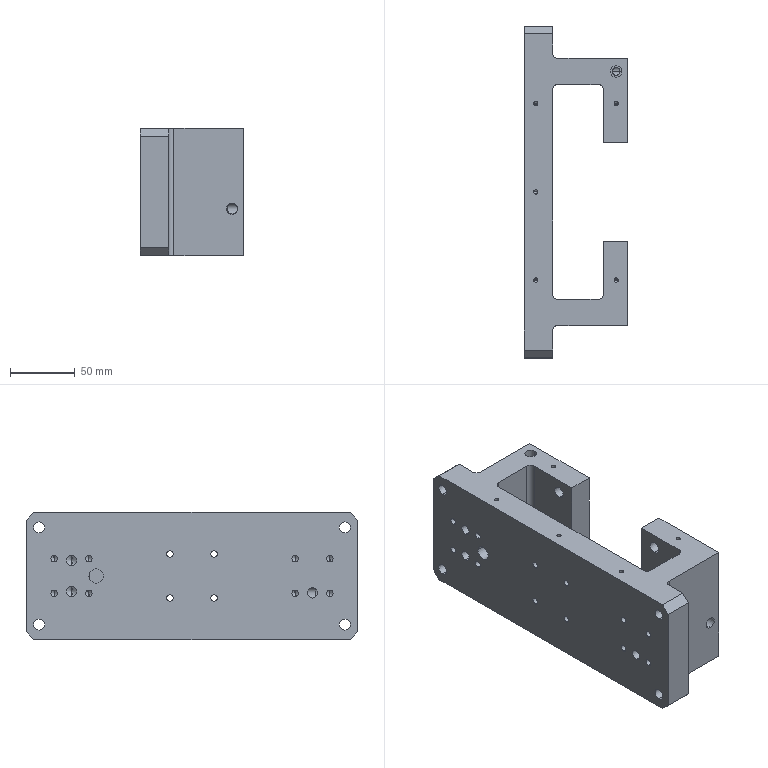Part | SolidWorks | features HoleWzd 16, MirrorPattern 3, 3DProfileFeature 2, Chamfer 1, CirPattern 1, Extrusion 1, Fillet 1, ICE 1 | 1 solid | 205 faces | box 80 x 256 x 98 mm | volume 906653 mm3 | cylinder 122 | cone 54 | plane 29 | commonest cylinder face diameters 5 x24 6 x22 3.3 x20 8 x20 8.5 x16 8.8 x10